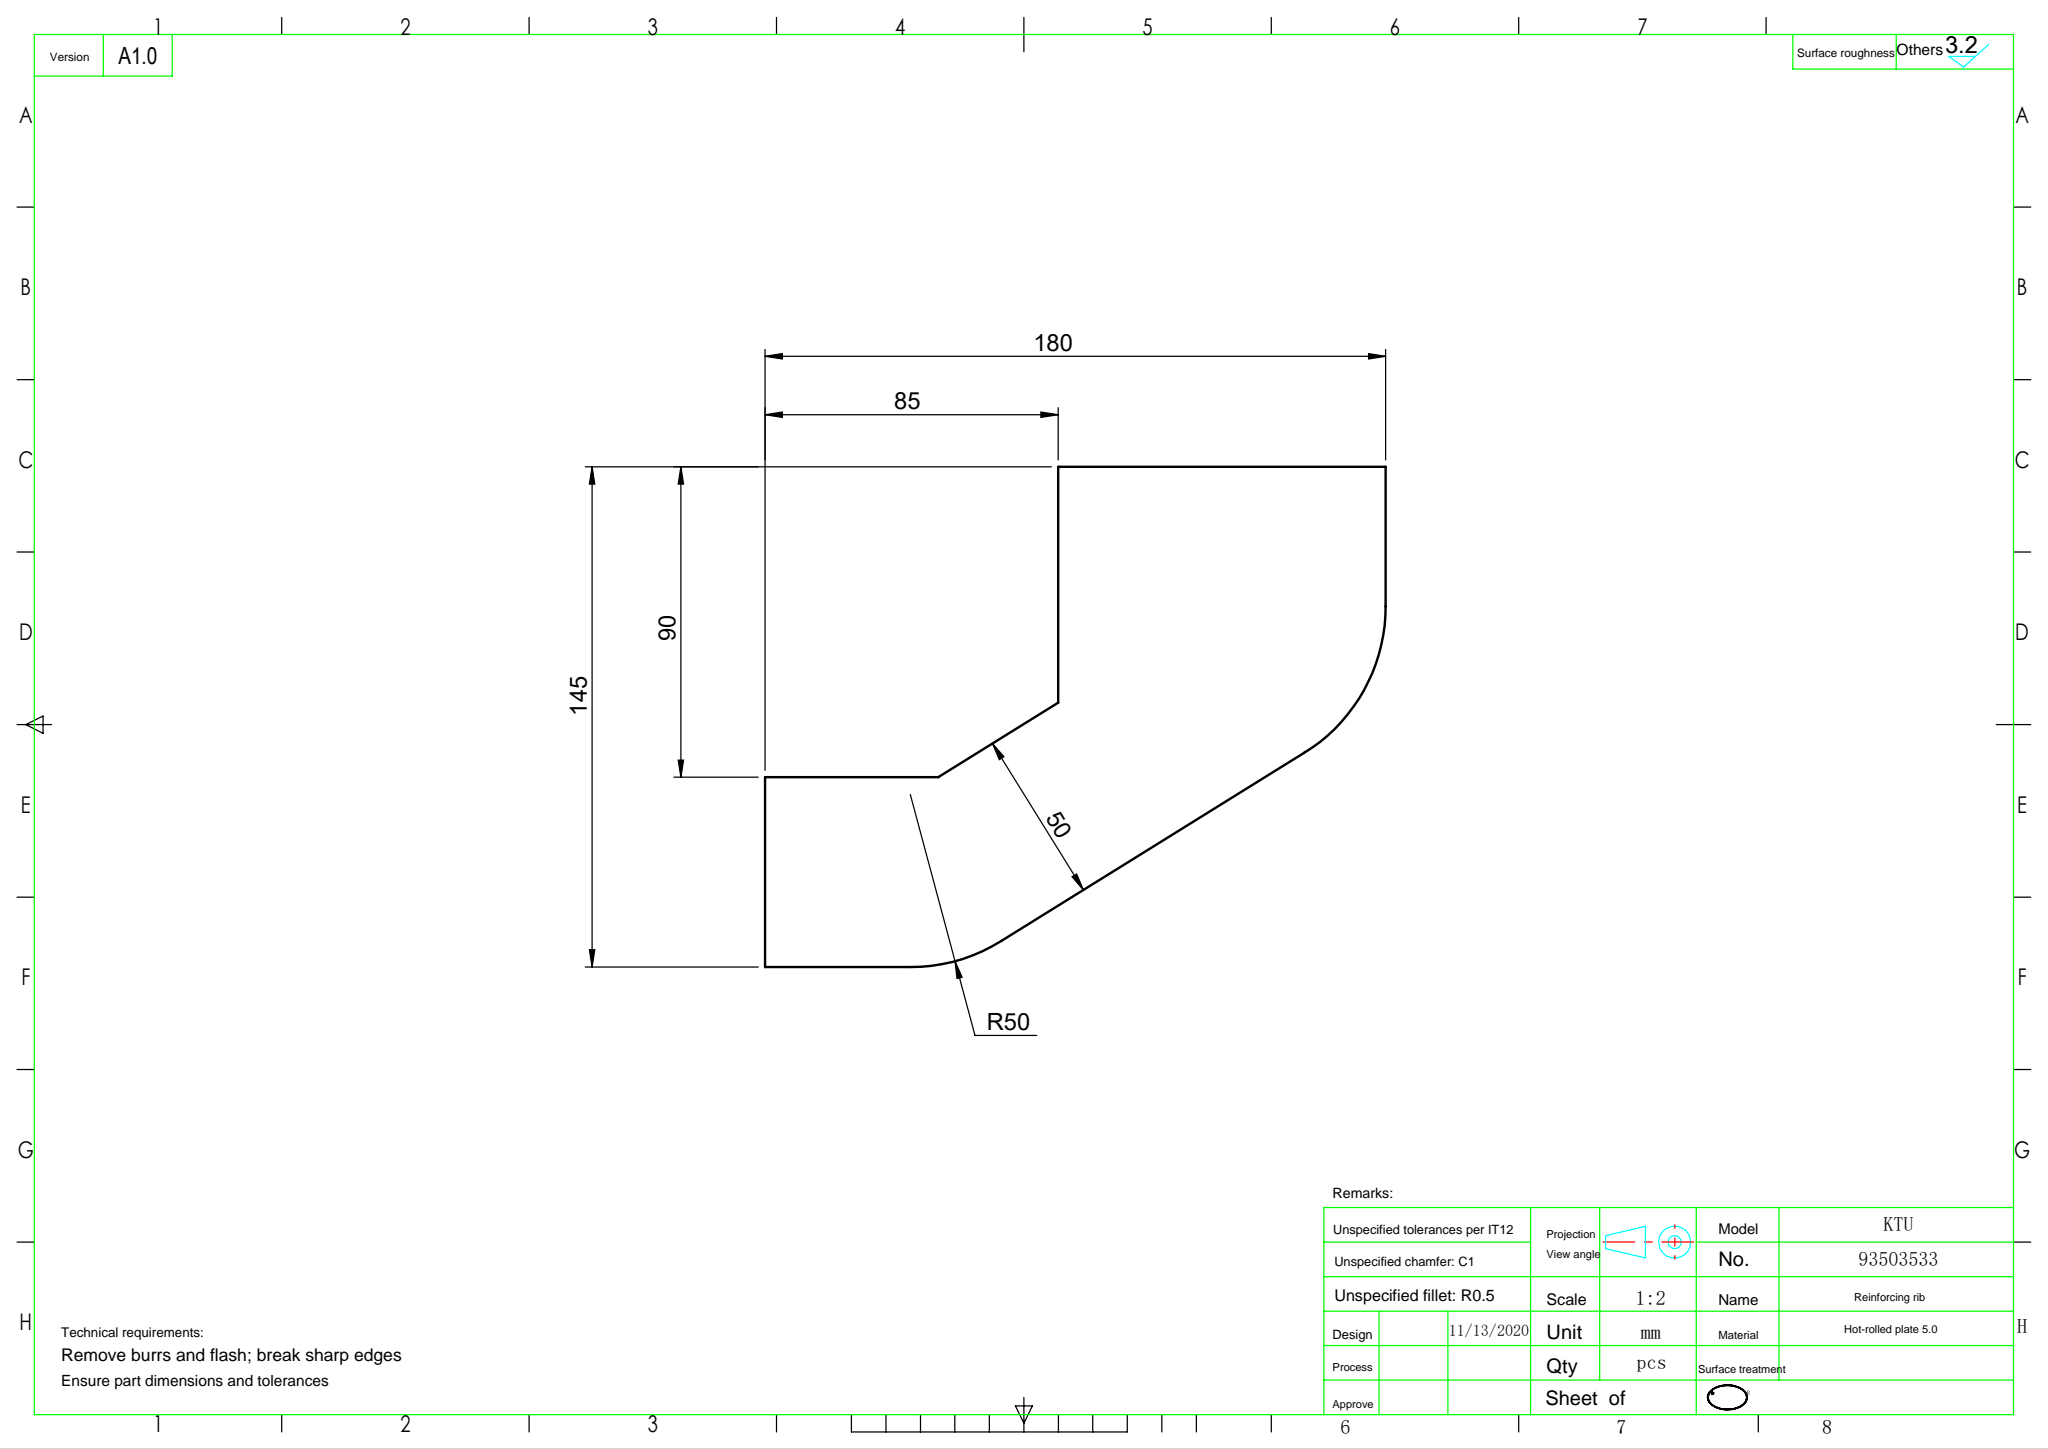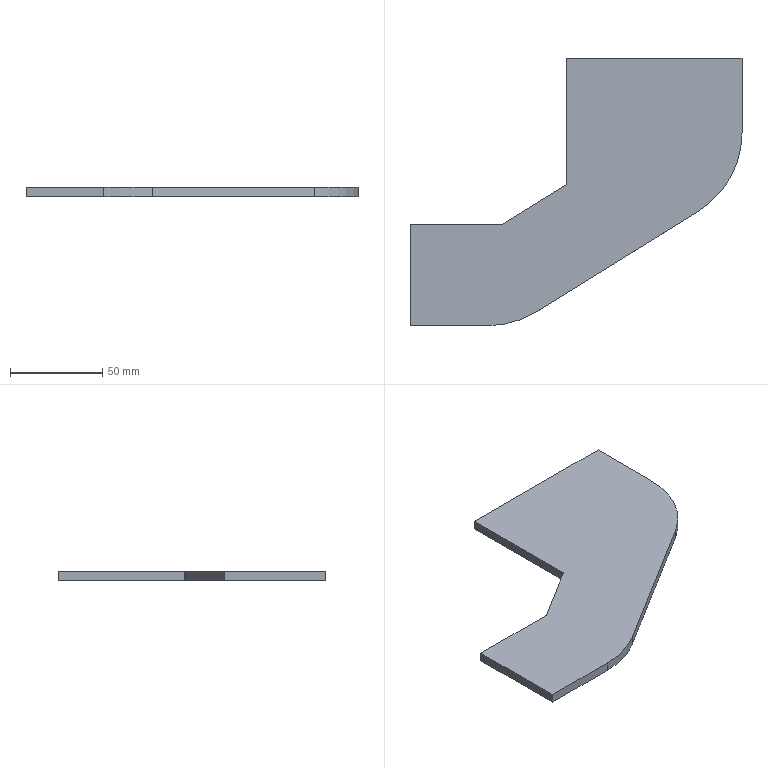Part | SolidWorks | features ICE 2, Fillet 1, FlatPattern 1, SMBaseFlange 1, SheetMetal 1 | 1 solid | 12 faces | box 180 x 145 x 5 mm | volume 69721 mm3 | plane 10 | cylinder 2 | commonest cylinder face diameters 100 x2
STEP:
#1=CARTESIAN_POINT('',(68.501,-137.482,-5.));
#2=VERTEX_POINT('',#1);
#3=CARTESIAN_POINT('',(156.368,-82.944,-5.));
#4=VERTEX_POINT('',#3);
#5=CARTESIAN_POINT('',(290.,0.,-5.));
#6=DIRECTION('',(0.8496,0.5274,0.));
#7=VECTOR('',#6,1000.);
#8=LINE('',#5,#7);
#9=EDGE_CURVE('',#2,#4,#8,.T.);
#10=ORIENTED_EDGE('',*,*,#9,.T.);
#11=CARTESIAN_POINT('',(156.368,-82.944,0.));
#12=VERTEX_POINT('',#11);
#13=CARTESIAN_POINT('',(156.368,-82.944,-5.));
#14=DIRECTION('',(0.,0.,1.));
#15=VECTOR('',#14,1000.);
#16=LINE('',#13,#15);
#17=EDGE_CURVE('',#4,#12,#16,.T.);
#18=ORIENTED_EDGE('',*,*,#17,.T.);
#19=CARTESIAN_POINT('',(68.501,-137.482,0.));
#20=VERTEX_POINT('',#19);
#21=CARTESIAN_POINT('',(290.,0.,0.));
#22=DIRECTION('',(0.8496,0.5274,0.));
#23=VECTOR('',#22,1000.);
#24=LINE('',#21,#23);
#25=EDGE_CURVE('',#20,#12,#24,.T.);
#26=ORIENTED_EDGE('',*,*,#25,.F.);
#27=CARTESIAN_POINT('',(68.501,-137.482,-5.));
#28=DIRECTION('',(0.,0.,-1.));
#29=VECTOR('',#28,1000.);
#30=LINE('',#27,#29);
#31=EDGE_CURVE('',#20,#2,#30,.T.);
#32=ORIENTED_EDGE('',*,*,#31,.T.);
#33=EDGE_LOOP('',(#10,#18,#26,#32));
#34=FACE_OUTER_BOUND('',#33,.T.);
#35=CARTESIAN_POINT('',(290.,0.,-5.));
#36=DIRECTION('',(0.5274,-0.8496,0.));
#37=DIRECTION('',(0.8496,0.5274,0.));
#38=AXIS2_PLACEMENT_3D('',#35,#36,#37);
#39=PLANE('',#38);
#40=ADVANCED_FACE('',(#34),#39,.T.);
#41=CARTESIAN_POINT('',(180.,0.,-5.));
#42=VERTEX_POINT('',#41);
#43=CARTESIAN_POINT('',(180.,-40.462,-5.));
#44=VERTEX_POINT('',#43);
#45=CARTESIAN_POINT('',(180.,0.,-5.));
#46=DIRECTION('',(0.,-1.,0.));
#47=VECTOR('',#46,1000.);
#48=LINE('',#45,#47);
#49=EDGE_CURVE('',#42,#44,#48,.T.);
#50=ORIENTED_EDGE('',*,*,#49,.T.);
#51=CARTESIAN_POINT('',(130.,-40.462,-5.));
#52=DIRECTION('',(0.,0.,-1.));
#53=DIRECTION('',(-1.,0.,0.));
#54=AXIS2_PLACEMENT_3D('',#51,#52,#53);
#55=CIRCLE('',#54,50.);
#56=EDGE_CURVE('',#44,#4,#55,.T.);
#57=ORIENTED_EDGE('',*,*,#56,.T.);
#58=ORIENTED_EDGE('',*,*,#9,.F.);
#59=CARTESIAN_POINT('',(42.133,-145.,-5.));
#60=VERTEX_POINT('',#59);
#61=CARTESIAN_POINT('',(42.133,-95.,-5.));
#62=DIRECTION('',(0.,0.,-1.));
#63=DIRECTION('',(-1.,0.,0.));
#64=AXIS2_PLACEMENT_3D('',#61,#62,#63);
#65=CIRCLE('',#64,50.);
#66=EDGE_CURVE('',#2,#60,#65,.T.);
#67=ORIENTED_EDGE('',*,*,#66,.T.);
#68=CARTESIAN_POINT('',(0.,-145.,-5.));
#69=VERTEX_POINT('',#68);
#70=CARTESIAN_POINT('',(0.,-145.,-5.));
#71=DIRECTION('',(-1.,0.,0.));
#72=VECTOR('',#71,1000.);
#73=LINE('',#70,#72);
#74=EDGE_CURVE('',#60,#69,#73,.T.);
#75=ORIENTED_EDGE('',*,*,#74,.T.);
#76=CARTESIAN_POINT('',(0.,-90.,-5.));
#77=VERTEX_POINT('',#76);
#78=CARTESIAN_POINT('',(0.,-180.,-5.));
#79=DIRECTION('',(0.,-1.,0.));
#80=VECTOR('',#79,1000.);
#81=LINE('',#78,#80);
#82=EDGE_CURVE('',#77,#69,#81,.T.);
#83=ORIENTED_EDGE('',*,*,#82,.F.);
#84=CARTESIAN_POINT('',(50.189,-90.,-5.));
#85=VERTEX_POINT('',#84);
#86=CARTESIAN_POINT('',(0.,-90.,-5.));
#87=DIRECTION('',(1.,0.,0.));
#88=VECTOR('',#87,1000.);
#89=LINE('',#86,#88);
#90=EDGE_CURVE('',#77,#85,#89,.T.);
#91=ORIENTED_EDGE('',*,*,#90,.T.);
#92=CARTESIAN_POINT('',(85.,-68.393,-5.));
#93=VERTEX_POINT('',#92);
#94=CARTESIAN_POINT('',(85.,-68.393,-5.));
#95=DIRECTION('',(0.8496,0.5274,0.));
#96=VECTOR('',#95,1000.);
#97=LINE('',#94,#96);
#98=EDGE_CURVE('',#85,#93,#97,.T.);
#99=ORIENTED_EDGE('',*,*,#98,.T.);
#100=CARTESIAN_POINT('',(85.,0.,-5.));
#101=VERTEX_POINT('',#100);
#102=CARTESIAN_POINT('',(85.,0.,-5.));
#103=DIRECTION('',(0.,1.,0.));
#104=VECTOR('',#103,1000.);
#105=LINE('',#102,#104);
#106=EDGE_CURVE('',#93,#101,#105,.T.);
#107=ORIENTED_EDGE('',*,*,#106,.T.);
#108=CARTESIAN_POINT('',(0.,0.,-5.));
#109=DIRECTION('',(-1.,0.,0.));
#110=VECTOR('',#109,1000.);
#111=LINE('',#108,#110);
#112=EDGE_CURVE('',#42,#101,#111,.T.);
#113=ORIENTED_EDGE('',*,*,#112,.F.);
#114=EDGE_LOOP('',(#50,#57,#58,#67,#75,#83,#91,#99,#107,#113));
#115=FACE_OUTER_BOUND('',#114,.T.);
#116=CARTESIAN_POINT('',(0.,0.,-5.));
#117=DIRECTION('',(0.,0.,-1.));
#118=DIRECTION('',(-1.,0.,0.));
#119=AXIS2_PLACEMENT_3D('',#116,#117,#118);
#120=PLANE('',#119);
#121=ADVANCED_FACE('',(#115),#120,.T.);
#122=ORIENTED_EDGE('',*,*,#25,.T.);
#123=CARTESIAN_POINT('',(180.,-40.462,0.));
#124=VERTEX_POINT('',#123);
#125=CARTESIAN_POINT('',(130.,-40.462,0.));
#126=DIRECTION('',(0.,0.,1.));
#127=DIRECTION('',(-1.,0.,0.));
#128=AXIS2_PLACEMENT_3D('',#125,#126,#127);
#129=CIRCLE('',#128,50.);
#130=EDGE_CURVE('',#12,#124,#129,.T.);
#131=ORIENTED_EDGE('',*,*,#130,.T.);
#132=CARTESIAN_POINT('',(180.,0.,0.));
#133=VERTEX_POINT('',#132);
#134=CARTESIAN_POINT('',(180.,0.,0.));
#135=DIRECTION('',(0.,-1.,0.));
#136=VECTOR('',#135,1000.);
#137=LINE('',#134,#136);
#138=EDGE_CURVE('',#133,#124,#137,.T.);
#139=ORIENTED_EDGE('',*,*,#138,.F.);
#140=CARTESIAN_POINT('',(85.,0.,0.));
#141=VERTEX_POINT('',#140);
#142=CARTESIAN_POINT('',(0.,0.,0.));
#143=DIRECTION('',(-1.,0.,0.));
#144=VECTOR('',#143,1000.);
#145=LINE('',#142,#144);
#146=EDGE_CURVE('',#133,#141,#145,.T.);
#147=ORIENTED_EDGE('',*,*,#146,.T.);
#148=CARTESIAN_POINT('',(85.,-68.393,0.));
#149=VERTEX_POINT('',#148);
#150=CARTESIAN_POINT('',(85.,0.,0.));
#151=DIRECTION('',(0.,1.,0.));
#152=VECTOR('',#151,1000.);
#153=LINE('',#150,#152);
#154=EDGE_CURVE('',#149,#141,#153,.T.);
#155=ORIENTED_EDGE('',*,*,#154,.F.);
#156=CARTESIAN_POINT('',(50.189,-90.,0.));
#157=VERTEX_POINT('',#156);
#158=CARTESIAN_POINT('',(85.,-68.393,0.));
#159=DIRECTION('',(0.8496,0.5274,0.));
#160=VECTOR('',#159,1000.);
#161=LINE('',#158,#160);
#162=EDGE_CURVE('',#157,#149,#161,.T.);
#163=ORIENTED_EDGE('',*,*,#162,.F.);
#164=CARTESIAN_POINT('',(0.,-90.,0.));
#165=VERTEX_POINT('',#164);
#166=CARTESIAN_POINT('',(0.,-90.,0.));
#167=DIRECTION('',(1.,0.,0.));
#168=VECTOR('',#167,1000.);
#169=LINE('',#166,#168);
#170=EDGE_CURVE('',#165,#157,#169,.T.);
#171=ORIENTED_EDGE('',*,*,#170,.F.);
#172=CARTESIAN_POINT('',(0.,-145.,0.));
#173=VERTEX_POINT('',#172);
#174=CARTESIAN_POINT('',(0.,-180.,0.));
#175=DIRECTION('',(0.,-1.,0.));
#176=VECTOR('',#175,1000.);
#177=LINE('',#174,#176);
#178=EDGE_CURVE('',#165,#173,#177,.T.);
#179=ORIENTED_EDGE('',*,*,#178,.T.);
#180=CARTESIAN_POINT('',(42.133,-145.,0.));
#181=VERTEX_POINT('',#180);
#182=CARTESIAN_POINT('',(0.,-145.,0.));
#183=DIRECTION('',(-1.,0.,0.));
#184=VECTOR('',#183,1000.);
#185=LINE('',#182,#184);
#186=EDGE_CURVE('',#181,#173,#185,.T.);
#187=ORIENTED_EDGE('',*,*,#186,.F.);
#188=CARTESIAN_POINT('',(42.133,-95.,0.));
#189=DIRECTION('',(0.,0.,1.));
#190=DIRECTION('',(-1.,0.,0.));
#191=AXIS2_PLACEMENT_3D('',#188,#189,#190);
#192=CIRCLE('',#191,50.);
#193=EDGE_CURVE('',#181,#20,#192,.T.);
#194=ORIENTED_EDGE('',*,*,#193,.T.);
#195=EDGE_LOOP('',(#122,#131,#139,#147,#155,#163,#171,#179,#187,#194));
#196=FACE_OUTER_BOUND('',#195,.T.);
#197=CARTESIAN_POINT('',(0.,0.,0.));
#198=DIRECTION('',(0.,0.,-1.));
#199=DIRECTION('',(-1.,0.,0.));
#200=AXIS2_PLACEMENT_3D('',#197,#198,#199);
#201=PLANE('',#200);
#202=ADVANCED_FACE('',(#196),#201,.F.);
#203=ORIENTED_EDGE('',*,*,#146,.F.);
#204=CARTESIAN_POINT('',(180.,0.,-5.));
#205=DIRECTION('',(0.,0.,1.));
#206=VECTOR('',#205,1000.);
#207=LINE('',#204,#206);
#208=EDGE_CURVE('',#42,#133,#207,.T.);
#209=ORIENTED_EDGE('',*,*,#208,.F.);
#210=ORIENTED_EDGE('',*,*,#112,.T.);
#211=CARTESIAN_POINT('',(85.,0.,-5.001));
#212=DIRECTION('',(0.,0.,1.));
#213=VECTOR('',#212,1000.);
#214=LINE('',#211,#213);
#215=EDGE_CURVE('',#101,#141,#214,.T.);
#216=ORIENTED_EDGE('',*,*,#215,.T.);
#217=EDGE_LOOP('',(#203,#209,#210,#216));
#218=FACE_OUTER_BOUND('',#217,.T.);
#219=CARTESIAN_POINT('',(0.,0.,-5.));
#220=DIRECTION('',(0.,1.,0.));
#221=DIRECTION('',(0.,0.,1.));
#222=AXIS2_PLACEMENT_3D('',#219,#220,#221);
#223=PLANE('',#222);
#224=ADVANCED_FACE('',(#218),#223,.T.);
#225=ORIENTED_EDGE('',*,*,#82,.T.);
#226=CARTESIAN_POINT('',(0.,-145.,-5.));
#227=DIRECTION('',(0.,0.,1.));
#228=VECTOR('',#227,1000.);
#229=LINE('',#226,#228);
#230=EDGE_CURVE('',#69,#173,#229,.T.);
#231=ORIENTED_EDGE('',*,*,#230,.T.);
#232=ORIENTED_EDGE('',*,*,#178,.F.);
#233=CARTESIAN_POINT('',(0.,-90.,-5.001));
#234=DIRECTION('',(0.,0.,1.));
#235=VECTOR('',#234,1000.);
#236=LINE('',#233,#235);
#237=EDGE_CURVE('',#77,#165,#236,.T.);
#238=ORIENTED_EDGE('',*,*,#237,.F.);
#239=EDGE_LOOP('',(#225,#231,#232,#238));
#240=FACE_OUTER_BOUND('',#239,.T.);
#241=CARTESIAN_POINT('',(0.,-180.,-5.));
#242=DIRECTION('',(-1.,0.,0.));
#243=DIRECTION('',(0.,0.,1.));
#244=AXIS2_PLACEMENT_3D('',#241,#242,#243);
#245=PLANE('',#244);
#246=ADVANCED_FACE('',(#240),#245,.T.);
#247=CARTESIAN_POINT('',(85.,-68.393,-5.001));
#248=DIRECTION('',(0.,0.,1.));
#249=VECTOR('',#248,1000.);
#250=LINE('',#247,#249);
#251=EDGE_CURVE('',#93,#149,#250,.T.);
#252=ORIENTED_EDGE('',*,*,#251,.T.);
#253=ORIENTED_EDGE('',*,*,#154,.T.);
#254=ORIENTED_EDGE('',*,*,#215,.F.);
#255=ORIENTED_EDGE('',*,*,#106,.F.);
#256=EDGE_LOOP('',(#252,#253,#254,#255));
#257=FACE_OUTER_BOUND('',#256,.T.);
#258=CARTESIAN_POINT('',(85.,0.,-5.001));
#259=DIRECTION('',(1.,0.,0.));
#260=DIRECTION('',(0.,1.,0.));
#261=AXIS2_PLACEMENT_3D('',#258,#259,#260);
#262=PLANE('',#261);
#263=ADVANCED_FACE('',(#257),#262,.F.);
#264=CARTESIAN_POINT('',(50.189,-90.,-5.001));
#265=DIRECTION('',(0.,0.,1.));
#266=VECTOR('',#265,1000.);
#267=LINE('',#264,#266);
#268=EDGE_CURVE('',#85,#157,#267,.T.);
#269=ORIENTED_EDGE('',*,*,#268,.T.);
#270=ORIENTED_EDGE('',*,*,#162,.T.);
#271=ORIENTED_EDGE('',*,*,#251,.F.);
#272=ORIENTED_EDGE('',*,*,#98,.F.);
#273=EDGE_LOOP('',(#269,#270,#271,#272));
#274=FACE_OUTER_BOUND('',#273,.T.);
#275=CARTESIAN_POINT('',(85.,-68.393,-5.001));
#276=DIRECTION('',(0.5274,-0.8496,0.));
#277=DIRECTION('',(0.8496,0.5274,0.));
#278=AXIS2_PLACEMENT_3D('',#275,#276,#277);
#279=PLANE('',#278);
#280=ADVANCED_FACE('',(#274),#279,.F.);
#281=ORIENTED_EDGE('',*,*,#237,.T.);
#282=ORIENTED_EDGE('',*,*,#170,.T.);
#283=ORIENTED_EDGE('',*,*,#268,.F.);
#284=ORIENTED_EDGE('',*,*,#90,.F.);
#285=EDGE_LOOP('',(#281,#282,#283,#284));
#286=FACE_OUTER_BOUND('',#285,.T.);
#287=CARTESIAN_POINT('',(0.,-90.,-5.001));
#288=DIRECTION('',(0.,-1.,0.));
#289=DIRECTION('',(0.,0.,-1.));
#290=AXIS2_PLACEMENT_3D('',#287,#288,#289);
#291=PLANE('',#290);
#292=ADVANCED_FACE('',(#286),#291,.F.);
#293=ORIENTED_EDGE('',*,*,#74,.F.);
#294=CARTESIAN_POINT('',(42.133,-145.,-5.));
#295=DIRECTION('',(0.,0.,1.));
#296=VECTOR('',#295,1000.);
#297=LINE('',#294,#296);
#298=EDGE_CURVE('',#60,#181,#297,.T.);
#299=ORIENTED_EDGE('',*,*,#298,.T.);
#300=ORIENTED_EDGE('',*,*,#186,.T.);
#301=ORIENTED_EDGE('',*,*,#230,.F.);
#302=EDGE_LOOP('',(#293,#299,#300,#301));
#303=FACE_OUTER_BOUND('',#302,.T.);
#304=CARTESIAN_POINT('',(0.,-145.,-5.));
#305=DIRECTION('',(0.,-1.,0.));
#306=DIRECTION('',(-1.,0.,0.));
#307=AXIS2_PLACEMENT_3D('',#304,#305,#306);
#308=PLANE('',#307);
#309=ADVANCED_FACE('',(#303),#308,.T.);
#310=ORIENTED_EDGE('',*,*,#138,.T.);
#311=CARTESIAN_POINT('',(180.,-40.462,-5.));
#312=DIRECTION('',(0.,0.,-1.));
#313=VECTOR('',#312,1000.);
#314=LINE('',#311,#313);
#315=EDGE_CURVE('',#124,#44,#314,.T.);
#316=ORIENTED_EDGE('',*,*,#315,.T.);
#317=ORIENTED_EDGE('',*,*,#49,.F.);
#318=ORIENTED_EDGE('',*,*,#208,.T.);
#319=EDGE_LOOP('',(#310,#316,#317,#318));
#320=FACE_OUTER_BOUND('',#319,.T.);
#321=CARTESIAN_POINT('',(180.,0.,-5.));
#322=DIRECTION('',(1.,0.,0.));
#323=DIRECTION('',(0.,-1.,0.));
#324=AXIS2_PLACEMENT_3D('',#321,#322,#323);
#325=PLANE('',#324);
#326=ADVANCED_FACE('',(#320),#325,.T.);
#327=ORIENTED_EDGE('',*,*,#56,.F.);
#328=ORIENTED_EDGE('',*,*,#315,.F.);
#329=ORIENTED_EDGE('',*,*,#130,.F.);
#330=ORIENTED_EDGE('',*,*,#17,.F.);
#331=EDGE_LOOP('',(#327,#328,#329,#330));
#332=FACE_OUTER_BOUND('',#331,.T.);
#333=CARTESIAN_POINT('',(130.,-40.462,-5.));
#334=DIRECTION('',(0.,0.,1.));
#335=DIRECTION('',(1.,0.,0.));
#336=AXIS2_PLACEMENT_3D('',#333,#334,#335);
#337=CYLINDRICAL_SURFACE('',#336,50.);
#338=ADVANCED_FACE('',(#332),#337,.T.);
#339=ORIENTED_EDGE('',*,*,#66,.F.);
#340=ORIENTED_EDGE('',*,*,#31,.F.);
#341=ORIENTED_EDGE('',*,*,#193,.F.);
#342=ORIENTED_EDGE('',*,*,#298,.F.);
#343=EDGE_LOOP('',(#339,#340,#341,#342));
#344=FACE_OUTER_BOUND('',#343,.T.);
#345=CARTESIAN_POINT('',(42.133,-95.,-5.));
#346=DIRECTION('',(0.,0.,1.));
#347=DIRECTION('',(1.,0.,0.));
#348=AXIS2_PLACEMENT_3D('',#345,#346,#347);
#349=CYLINDRICAL_SURFACE('',#348,50.);
#350=ADVANCED_FACE('',(#344),#349,.T.);
#351=CLOSED_SHELL('',(#40,#121,#202,#224,#246,#263,#280,#292,#309,#326,#338,#350));
#352=MANIFOLD_SOLID_BREP('',#351);
#353=CARTESIAN_POINT('',(0.,0.,0.));
#354=DIRECTION('',(0.,0.,1.));
#355=DIRECTION('',(1.,0.,0.));
#356=AXIS2_PLACEMENT_3D('',#353,#354,#355);
#357=(LENGTH_UNIT()NAMED_UNIT(*)SI_UNIT(.MILLI.,.METRE.));
#358=UNCERTAINTY_MEASURE_WITH_UNIT(LENGTH_MEASURE(0.00001),#357,'','');
#359=(NAMED_UNIT(*)PLANE_ANGLE_UNIT()SI_UNIT($,.RADIAN.));
#360=(NAMED_UNIT(*)SI_UNIT($,.STERADIAN.)SOLID_ANGLE_UNIT());
#361=(GEOMETRIC_REPRESENTATION_CONTEXT(3)GLOBAL_UNCERTAINTY_ASSIGNED_CONTEXT((#358))GLOBAL_UNIT_ASSIGNED_CONTEXT((#357,#359,#360))REPRESENTATION_CONTEXT('',''));
#362=ADVANCED_BREP_SHAPE_REPRESENTATION('',(#352,#356),#361);